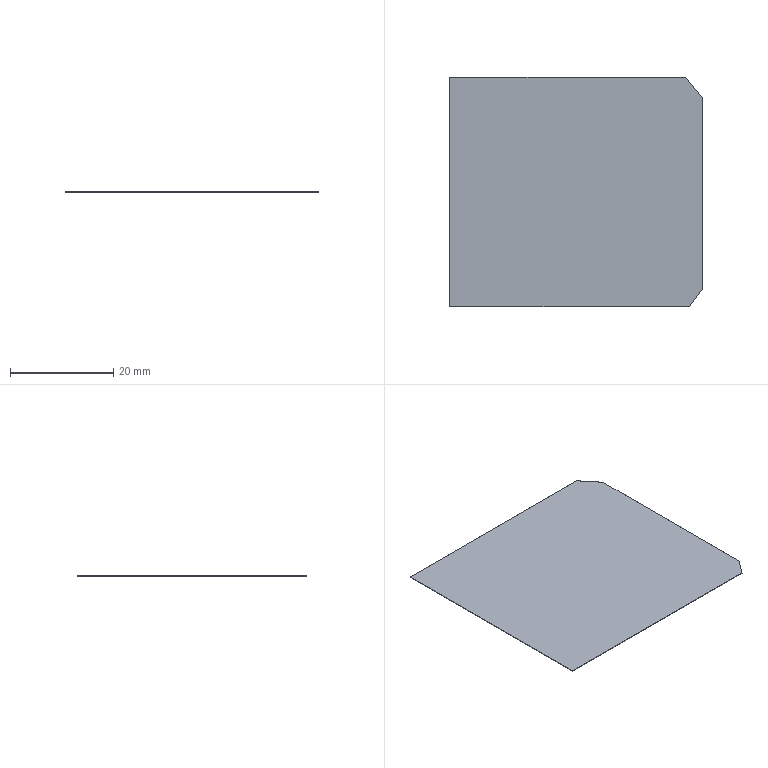Part | NX | features DATUM_CSYS 2, EXTRUDE 1, SKETCH 1 | 1 solid | 8 faces | box 48.88 x 44.5 x 0.1 mm | volume 216.462 mm3 | plane 8
STEP:
#1=CARTESIAN_POINT('',(0.,44.5,0.));
#2=VERTEX_POINT('',#1);
#3=CARTESIAN_POINT('',(0.,0.,0.));
#4=VERTEX_POINT('',#3);
#5=CARTESIAN_POINT('',(0.,44.5,0.));
#6=DIRECTION('',(0.,-1.,0.));
#7=VECTOR('',#6,1000.);
#8=LINE('',#5,#7);
#9=EDGE_CURVE('',#2,#4,#8,.T.);
#10=ORIENTED_EDGE('',*,*,#9,.T.);
#11=CARTESIAN_POINT('',(0.,0.,0.1));
#12=VERTEX_POINT('',#11);
#13=CARTESIAN_POINT('',(0.,0.,0.1));
#14=DIRECTION('',(0.,0.,-1.));
#15=VECTOR('',#14,1000.);
#16=LINE('',#13,#15);
#17=EDGE_CURVE('',#12,#4,#16,.T.);
#18=ORIENTED_EDGE('',*,*,#17,.F.);
#19=CARTESIAN_POINT('',(0.,44.5,0.1));
#20=VERTEX_POINT('',#19);
#21=CARTESIAN_POINT('',(0.,44.5,0.1));
#22=DIRECTION('',(0.,-1.,0.));
#23=VECTOR('',#22,1000.);
#24=LINE('',#21,#23);
#25=EDGE_CURVE('',#20,#12,#24,.T.);
#26=ORIENTED_EDGE('',*,*,#25,.F.);
#27=CARTESIAN_POINT('',(0.,44.5,0.1));
#28=DIRECTION('',(0.,0.,-1.));
#29=VECTOR('',#28,1000.);
#30=LINE('',#27,#29);
#31=EDGE_CURVE('',#20,#2,#30,.T.);
#32=ORIENTED_EDGE('',*,*,#31,.T.);
#33=EDGE_LOOP('',(#10,#18,#26,#32));
#34=FACE_BOUND('',#33,.T.);
#35=CARTESIAN_POINT('',(0.,44.5,0.1));
#36=DIRECTION('',(1.,0.,0.));
#37=DIRECTION('',(0.,1.,0.));
#38=AXIS2_PLACEMENT_3D('',#35,#36,#37);
#39=PLANE('',#38);
#40=ADVANCED_FACE('',(#34),#39,.F.);
#41=CARTESIAN_POINT('',(46.39,0.,0.));
#42=VERTEX_POINT('',#41);
#43=CARTESIAN_POINT('',(0.,0.,0.));
#44=DIRECTION('',(1.,0.,0.));
#45=VECTOR('',#44,1000.);
#46=LINE('',#43,#45);
#47=EDGE_CURVE('',#4,#42,#46,.T.);
#48=ORIENTED_EDGE('',*,*,#47,.T.);
#49=CARTESIAN_POINT('',(46.39,0.,0.1));
#50=VERTEX_POINT('',#49);
#51=CARTESIAN_POINT('',(46.39,0.,0.1));
#52=DIRECTION('',(0.,0.,-1.));
#53=VECTOR('',#52,1000.);
#54=LINE('',#51,#53);
#55=EDGE_CURVE('',#50,#42,#54,.T.);
#56=ORIENTED_EDGE('',*,*,#55,.F.);
#57=CARTESIAN_POINT('',(0.,0.,0.1));
#58=DIRECTION('',(1.,0.,0.));
#59=VECTOR('',#58,1000.);
#60=LINE('',#57,#59);
#61=EDGE_CURVE('',#12,#50,#60,.T.);
#62=ORIENTED_EDGE('',*,*,#61,.F.);
#63=ORIENTED_EDGE('',*,*,#17,.T.);
#64=EDGE_LOOP('',(#48,#56,#62,#63));
#65=FACE_BOUND('',#64,.T.);
#66=CARTESIAN_POINT('',(0.,0.,0.1));
#67=DIRECTION('',(0.,1.,0.));
#68=DIRECTION('',(0.,0.,1.));
#69=AXIS2_PLACEMENT_3D('',#66,#67,#68);
#70=PLANE('',#69);
#71=ADVANCED_FACE('',(#65),#70,.F.);
#72=CARTESIAN_POINT('',(48.88,3.35,0.));
#73=VERTEX_POINT('',#72);
#74=CARTESIAN_POINT('',(46.39,0.,0.));
#75=DIRECTION('',(0.5965,0.8026,0.));
#76=VECTOR('',#75,1000.);
#77=LINE('',#74,#76);
#78=EDGE_CURVE('',#42,#73,#77,.T.);
#79=ORIENTED_EDGE('',*,*,#78,.T.);
#80=CARTESIAN_POINT('',(48.88,3.35,0.1));
#81=VERTEX_POINT('',#80);
#82=CARTESIAN_POINT('',(48.88,3.35,0.1));
#83=DIRECTION('',(0.,0.,-1.));
#84=VECTOR('',#83,1000.);
#85=LINE('',#82,#84);
#86=EDGE_CURVE('',#81,#73,#85,.T.);
#87=ORIENTED_EDGE('',*,*,#86,.F.);
#88=CARTESIAN_POINT('',(46.39,0.,0.1));
#89=DIRECTION('',(0.5965,0.8026,0.));
#90=VECTOR('',#89,1000.);
#91=LINE('',#88,#90);
#92=EDGE_CURVE('',#50,#81,#91,.T.);
#93=ORIENTED_EDGE('',*,*,#92,.F.);
#94=ORIENTED_EDGE('',*,*,#55,.T.);
#95=EDGE_LOOP('',(#79,#87,#93,#94));
#96=FACE_BOUND('',#95,.T.);
#97=CARTESIAN_POINT('',(46.39,0.,0.1));
#98=DIRECTION('',(-0.8026,0.5965,0.));
#99=DIRECTION('',(-0.5965,-0.8026,0.));
#100=AXIS2_PLACEMENT_3D('',#97,#98,#99);
#101=PLANE('',#100);
#102=ADVANCED_FACE('',(#96),#101,.F.);
#103=CARTESIAN_POINT('',(48.88,40.57,0.));
#104=VERTEX_POINT('',#103);
#105=CARTESIAN_POINT('',(48.88,3.35,0.));
#106=DIRECTION('',(0.,1.,0.));
#107=VECTOR('',#106,1000.);
#108=LINE('',#105,#107);
#109=EDGE_CURVE('',#73,#104,#108,.T.);
#110=ORIENTED_EDGE('',*,*,#109,.T.);
#111=CARTESIAN_POINT('',(48.88,40.57,0.1));
#112=VERTEX_POINT('',#111);
#113=CARTESIAN_POINT('',(48.88,40.57,0.1));
#114=DIRECTION('',(0.,0.,-1.));
#115=VECTOR('',#114,1000.);
#116=LINE('',#113,#115);
#117=EDGE_CURVE('',#112,#104,#116,.T.);
#118=ORIENTED_EDGE('',*,*,#117,.F.);
#119=CARTESIAN_POINT('',(48.88,3.35,0.1));
#120=DIRECTION('',(0.,1.,0.));
#121=VECTOR('',#120,1000.);
#122=LINE('',#119,#121);
#123=EDGE_CURVE('',#81,#112,#122,.T.);
#124=ORIENTED_EDGE('',*,*,#123,.F.);
#125=ORIENTED_EDGE('',*,*,#86,.T.);
#126=EDGE_LOOP('',(#110,#118,#124,#125));
#127=FACE_BOUND('',#126,.T.);
#128=CARTESIAN_POINT('',(48.88,3.35,0.1));
#129=DIRECTION('',(-1.,0.,0.));
#130=DIRECTION('',(0.,-1.,0.));
#131=AXIS2_PLACEMENT_3D('',#128,#129,#130);
#132=PLANE('',#131);
#133=ADVANCED_FACE('',(#127),#132,.F.);
#134=CARTESIAN_POINT('',(45.64,44.5,0.));
#135=VERTEX_POINT('',#134);
#136=CARTESIAN_POINT('',(48.88,40.57,0.));
#137=DIRECTION('',(-0.6361,0.7716,0.));
#138=VECTOR('',#137,1000.);
#139=LINE('',#136,#138);
#140=EDGE_CURVE('',#104,#135,#139,.T.);
#141=ORIENTED_EDGE('',*,*,#140,.T.);
#142=CARTESIAN_POINT('',(45.64,44.5,0.1));
#143=VERTEX_POINT('',#142);
#144=CARTESIAN_POINT('',(45.64,44.5,0.1));
#145=DIRECTION('',(0.,0.,-1.));
#146=VECTOR('',#145,1000.);
#147=LINE('',#144,#146);
#148=EDGE_CURVE('',#143,#135,#147,.T.);
#149=ORIENTED_EDGE('',*,*,#148,.F.);
#150=CARTESIAN_POINT('',(48.88,40.57,0.1));
#151=DIRECTION('',(-0.6361,0.7716,0.));
#152=VECTOR('',#151,1000.);
#153=LINE('',#150,#152);
#154=EDGE_CURVE('',#112,#143,#153,.T.);
#155=ORIENTED_EDGE('',*,*,#154,.F.);
#156=ORIENTED_EDGE('',*,*,#117,.T.);
#157=EDGE_LOOP('',(#141,#149,#155,#156));
#158=FACE_BOUND('',#157,.T.);
#159=CARTESIAN_POINT('',(48.88,40.57,0.1));
#160=DIRECTION('',(-0.7716,-0.6361,0.));
#161=DIRECTION('',(0.6361,-0.7716,0.));
#162=AXIS2_PLACEMENT_3D('',#159,#160,#161);
#163=PLANE('',#162);
#164=ADVANCED_FACE('',(#158),#163,.F.);
#165=CARTESIAN_POINT('',(45.64,44.5,0.));
#166=DIRECTION('',(-1.,0.,0.));
#167=VECTOR('',#166,1000.);
#168=LINE('',#165,#167);
#169=EDGE_CURVE('',#135,#2,#168,.T.);
#170=ORIENTED_EDGE('',*,*,#169,.T.);
#171=ORIENTED_EDGE('',*,*,#31,.F.);
#172=CARTESIAN_POINT('',(45.64,44.5,0.1));
#173=DIRECTION('',(-1.,0.,0.));
#174=VECTOR('',#173,1000.);
#175=LINE('',#172,#174);
#176=EDGE_CURVE('',#143,#20,#175,.T.);
#177=ORIENTED_EDGE('',*,*,#176,.F.);
#178=ORIENTED_EDGE('',*,*,#148,.T.);
#179=EDGE_LOOP('',(#170,#171,#177,#178));
#180=FACE_BOUND('',#179,.T.);
#181=CARTESIAN_POINT('',(45.64,44.5,0.1));
#182=DIRECTION('',(0.,-1.,0.));
#183=DIRECTION('',(1.,0.,0.));
#184=AXIS2_PLACEMENT_3D('',#181,#182,#183);
#185=PLANE('',#184);
#186=ADVANCED_FACE('',(#180),#185,.F.);
#187=ORIENTED_EDGE('',*,*,#25,.T.);
#188=ORIENTED_EDGE('',*,*,#61,.T.);
#189=ORIENTED_EDGE('',*,*,#92,.T.);
#190=ORIENTED_EDGE('',*,*,#123,.T.);
#191=ORIENTED_EDGE('',*,*,#154,.T.);
#192=ORIENTED_EDGE('',*,*,#176,.T.);
#193=EDGE_LOOP('',(#187,#188,#189,#190,#191,#192));
#194=FACE_BOUND('',#193,.T.);
#195=CARTESIAN_POINT('',(0.,0.,0.1));
#196=DIRECTION('',(0.,0.,1.));
#197=DIRECTION('',(1.,0.,0.));
#198=AXIS2_PLACEMENT_3D('',#195,#196,#197);
#199=PLANE('',#198);
#200=ADVANCED_FACE('',(#194),#199,.T.);
#201=ORIENTED_EDGE('',*,*,#9,.F.);
#202=ORIENTED_EDGE('',*,*,#169,.F.);
#203=ORIENTED_EDGE('',*,*,#140,.F.);
#204=ORIENTED_EDGE('',*,*,#109,.F.);
#205=ORIENTED_EDGE('',*,*,#78,.F.);
#206=ORIENTED_EDGE('',*,*,#47,.F.);
#207=EDGE_LOOP('',(#201,#202,#203,#204,#205,#206));
#208=FACE_BOUND('',#207,.T.);
#209=CARTESIAN_POINT('',(0.,0.,0.));
#210=DIRECTION('',(0.,0.,1.));
#211=DIRECTION('',(1.,0.,0.));
#212=AXIS2_PLACEMENT_3D('',#209,#210,#211);
#213=PLANE('',#212);
#214=ADVANCED_FACE('',(#208),#213,.F.);
#215=CLOSED_SHELL('',(#40,#71,#102,#133,#164,#186,#200,#214));
#216=MANIFOLD_SOLID_BREP('',#215);
#217=(LENGTH_UNIT()NAMED_UNIT(*)SI_UNIT(.MILLI.,.METRE.));
#218=UNCERTAINTY_MEASURE_WITH_UNIT(LENGTH_MEASURE(0.00001),#217,'','');
#219=(NAMED_UNIT(*)PLANE_ANGLE_UNIT()SI_UNIT($,.RADIAN.));
#220=(NAMED_UNIT(*)SI_UNIT($,.STERADIAN.)SOLID_ANGLE_UNIT());
#221=(GEOMETRIC_REPRESENTATION_CONTEXT(3)GLOBAL_UNCERTAINTY_ASSIGNED_CONTEXT((#218))GLOBAL_UNIT_ASSIGNED_CONTEXT((#217,#219,#220))REPRESENTATION_CONTEXT('',''));
#222=ADVANCED_BREP_SHAPE_REPRESENTATION('',(#216),#221);